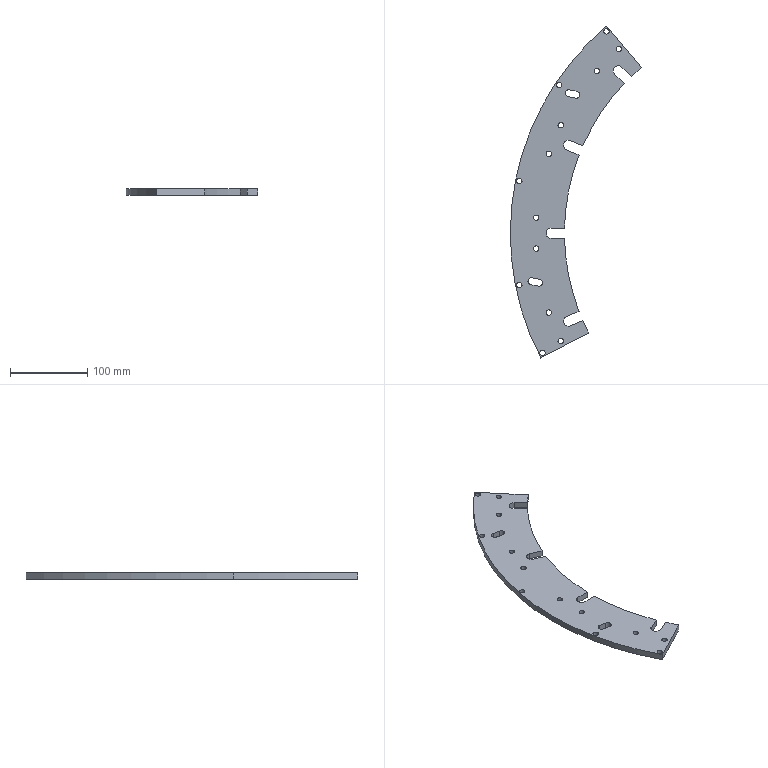Part | 1 solid | 59 faces | box 169.915 x 429.467 x 8 mm | volume 222646 mm3 | cylinder 43 | plane 16 | commonest cylinder face diameters 7 x26 9 x6 560 x5 13 x4 700 x2